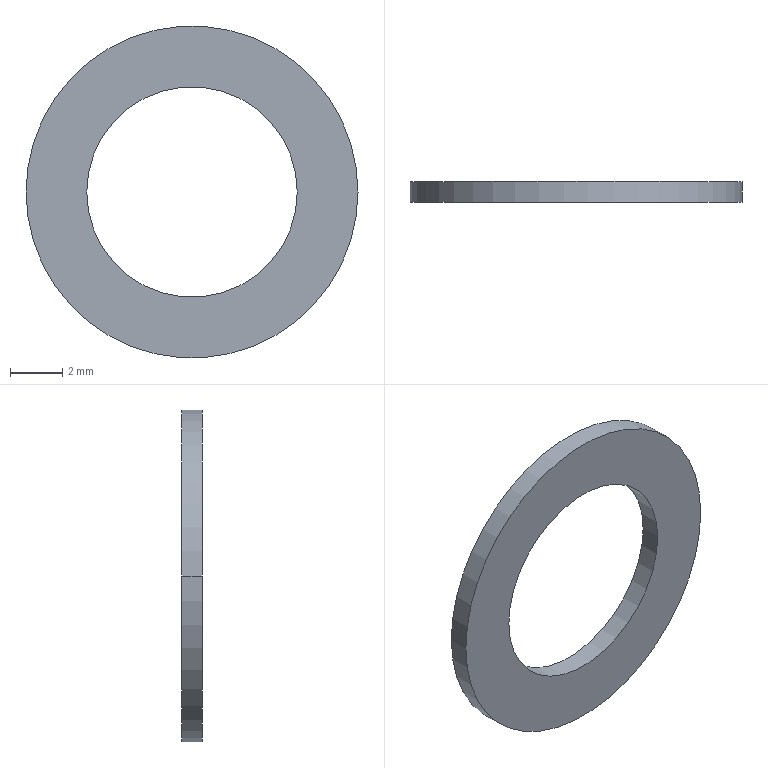Part | NX | features BREP 1 | 1 solid | 6 faces | box 12.7 x 0.7874 x 12.7 mm | volume 59.652 mm3 | cylinder 4 | plane 2 | commonest cylinder face diameters 8.052 x2 12.7 x2
STEP:
#1=CARTESIAN_POINT('',(-6.35,0.,0.));
#2=VERTEX_POINT('',#1);
#3=CARTESIAN_POINT('',(6.35,0.,0.));
#4=VERTEX_POINT('',#3);
#5=CARTESIAN_POINT('',(0.,0.,0.));
#6=DIRECTION('',(0.,1.,0.));
#7=DIRECTION('',(-1.,0.,0.));
#8=AXIS2_PLACEMENT_3D('',#5,#6,#7);
#9=CIRCLE('',#8,6.35);
#10=EDGE_CURVE('',#2,#4,#9,.T.);
#11=ORIENTED_EDGE('',*,*,#10,.F.);
#12=CARTESIAN_POINT('',(0.,0.,0.));
#13=DIRECTION('',(0.,1.,0.));
#14=DIRECTION('',(1.,0.,0.));
#15=AXIS2_PLACEMENT_3D('',#12,#13,#14);
#16=CIRCLE('',#15,6.35);
#17=EDGE_CURVE('',#4,#2,#16,.T.);
#18=ORIENTED_EDGE('',*,*,#17,.F.);
#19=EDGE_LOOP('',(#11,#18));
#20=FACE_BOUND('',#19,.T.);
#21=CARTESIAN_POINT('',(-4.026,0.,0.));
#22=VERTEX_POINT('',#21);
#23=CARTESIAN_POINT('',(4.026,0.,0.));
#24=VERTEX_POINT('',#23);
#25=CARTESIAN_POINT('',(0.,0.,0.));
#26=DIRECTION('',(0.,-1.,0.));
#27=DIRECTION('',(-1.,0.,0.));
#28=AXIS2_PLACEMENT_3D('',#25,#26,#27);
#29=CIRCLE('',#28,4.026);
#30=EDGE_CURVE('',#22,#24,#29,.T.);
#31=ORIENTED_EDGE('',*,*,#30,.F.);
#32=CARTESIAN_POINT('',(0.,0.,0.));
#33=DIRECTION('',(0.,-1.,0.));
#34=DIRECTION('',(1.,0.,0.));
#35=AXIS2_PLACEMENT_3D('',#32,#33,#34);
#36=CIRCLE('',#35,4.026);
#37=EDGE_CURVE('',#24,#22,#36,.T.);
#38=ORIENTED_EDGE('',*,*,#37,.F.);
#39=EDGE_LOOP('',(#31,#38));
#40=FACE_BOUND('',#39,.T.);
#41=CARTESIAN_POINT('',(0.,0.,0.));
#42=DIRECTION('',(0.,1.,0.));
#43=DIRECTION('',(1.,0.,0.));
#44=AXIS2_PLACEMENT_3D('',#41,#42,#43);
#45=PLANE('',#44);
#46=ADVANCED_FACE('',(#20,#40),#45,.F.);
#47=CARTESIAN_POINT('',(-6.35,0.7874,0.));
#48=VERTEX_POINT('',#47);
#49=CARTESIAN_POINT('',(-6.35,0.,0.));
#50=DIRECTION('',(0.,1.,0.));
#51=VECTOR('',#50,1000.);
#52=LINE('',#49,#51);
#53=EDGE_CURVE('',#2,#48,#52,.T.);
#54=ORIENTED_EDGE('',*,*,#53,.T.);
#55=CARTESIAN_POINT('',(6.35,0.7874,0.));
#56=VERTEX_POINT('',#55);
#57=CARTESIAN_POINT('',(0.,0.7874,0.));
#58=DIRECTION('',(0.,1.,0.));
#59=DIRECTION('',(1.,0.,0.));
#60=AXIS2_PLACEMENT_3D('',#57,#58,#59);
#61=CIRCLE('',#60,6.35);
#62=EDGE_CURVE('',#56,#48,#61,.T.);
#63=ORIENTED_EDGE('',*,*,#62,.F.);
#64=CARTESIAN_POINT('',(6.35,0.,0.));
#65=DIRECTION('',(0.,1.,0.));
#66=VECTOR('',#65,1000.);
#67=LINE('',#64,#66);
#68=EDGE_CURVE('',#4,#56,#67,.T.);
#69=ORIENTED_EDGE('',*,*,#68,.F.);
#70=ORIENTED_EDGE('',*,*,#17,.T.);
#71=EDGE_LOOP('',(#54,#63,#69,#70));
#72=FACE_BOUND('',#71,.T.);
#73=CARTESIAN_POINT('',(0.,0.,0.));
#74=DIRECTION('',(0.,1.,0.));
#75=DIRECTION('',(1.,0.,0.));
#76=AXIS2_PLACEMENT_3D('',#73,#74,#75);
#77=CYLINDRICAL_SURFACE('',#76,6.35);
#78=ADVANCED_FACE('',(#72),#77,.T.);
#79=ORIENTED_EDGE('',*,*,#68,.T.);
#80=CARTESIAN_POINT('',(0.,0.7874,0.));
#81=DIRECTION('',(0.,1.,0.));
#82=DIRECTION('',(-1.,0.,0.));
#83=AXIS2_PLACEMENT_3D('',#80,#81,#82);
#84=CIRCLE('',#83,6.35);
#85=EDGE_CURVE('',#48,#56,#84,.T.);
#86=ORIENTED_EDGE('',*,*,#85,.F.);
#87=ORIENTED_EDGE('',*,*,#53,.F.);
#88=ORIENTED_EDGE('',*,*,#10,.T.);
#89=EDGE_LOOP('',(#79,#86,#87,#88));
#90=FACE_BOUND('',#89,.T.);
#91=CARTESIAN_POINT('',(0.,0.,0.));
#92=DIRECTION('',(0.,1.,0.));
#93=DIRECTION('',(1.,0.,0.));
#94=AXIS2_PLACEMENT_3D('',#91,#92,#93);
#95=CYLINDRICAL_SURFACE('',#94,6.35);
#96=ADVANCED_FACE('',(#90),#95,.T.);
#97=ORIENTED_EDGE('',*,*,#85,.T.);
#98=ORIENTED_EDGE('',*,*,#62,.T.);
#99=EDGE_LOOP('',(#97,#98));
#100=FACE_BOUND('',#99,.T.);
#101=CARTESIAN_POINT('',(-4.026,0.7874,0.));
#102=VERTEX_POINT('',#101);
#103=CARTESIAN_POINT('',(4.026,0.7874,0.));
#104=VERTEX_POINT('',#103);
#105=CARTESIAN_POINT('',(0.,0.7874,0.));
#106=DIRECTION('',(0.,-1.,0.));
#107=DIRECTION('',(-1.,0.,0.));
#108=AXIS2_PLACEMENT_3D('',#105,#106,#107);
#109=CIRCLE('',#108,4.026);
#110=EDGE_CURVE('',#102,#104,#109,.T.);
#111=ORIENTED_EDGE('',*,*,#110,.T.);
#112=CARTESIAN_POINT('',(0.,0.7874,0.));
#113=DIRECTION('',(0.,-1.,0.));
#114=DIRECTION('',(1.,0.,0.));
#115=AXIS2_PLACEMENT_3D('',#112,#113,#114);
#116=CIRCLE('',#115,4.026);
#117=EDGE_CURVE('',#104,#102,#116,.T.);
#118=ORIENTED_EDGE('',*,*,#117,.T.);
#119=EDGE_LOOP('',(#111,#118));
#120=FACE_BOUND('',#119,.T.);
#121=CARTESIAN_POINT('',(0.,0.7874,0.));
#122=DIRECTION('',(0.,1.,0.));
#123=DIRECTION('',(1.,0.,0.));
#124=AXIS2_PLACEMENT_3D('',#121,#122,#123);
#125=PLANE('',#124);
#126=ADVANCED_FACE('',(#100,#120),#125,.T.);
#127=CARTESIAN_POINT('',(-4.026,0.7874,0.));
#128=DIRECTION('',(0.,-1.,0.));
#129=VECTOR('',#128,1000.);
#130=LINE('',#127,#129);
#131=EDGE_CURVE('',#102,#22,#130,.T.);
#132=ORIENTED_EDGE('',*,*,#131,.F.);
#133=ORIENTED_EDGE('',*,*,#117,.F.);
#134=CARTESIAN_POINT('',(4.026,0.7874,0.));
#135=DIRECTION('',(0.,-1.,0.));
#136=VECTOR('',#135,1000.);
#137=LINE('',#134,#136);
#138=EDGE_CURVE('',#104,#24,#137,.T.);
#139=ORIENTED_EDGE('',*,*,#138,.T.);
#140=ORIENTED_EDGE('',*,*,#37,.T.);
#141=EDGE_LOOP('',(#132,#133,#139,#140));
#142=FACE_BOUND('',#141,.T.);
#143=CARTESIAN_POINT('',(0.,0.7874,0.));
#144=DIRECTION('',(0.,-1.,0.));
#145=DIRECTION('',(1.,0.,0.));
#146=AXIS2_PLACEMENT_3D('',#143,#144,#145);
#147=CYLINDRICAL_SURFACE('',#146,4.026);
#148=ADVANCED_FACE('',(#142),#147,.F.);
#149=ORIENTED_EDGE('',*,*,#138,.F.);
#150=ORIENTED_EDGE('',*,*,#110,.F.);
#151=ORIENTED_EDGE('',*,*,#131,.T.);
#152=ORIENTED_EDGE('',*,*,#30,.T.);
#153=EDGE_LOOP('',(#149,#150,#151,#152));
#154=FACE_BOUND('',#153,.T.);
#155=CARTESIAN_POINT('',(0.,0.7874,0.));
#156=DIRECTION('',(0.,-1.,0.));
#157=DIRECTION('',(1.,0.,0.));
#158=AXIS2_PLACEMENT_3D('',#155,#156,#157);
#159=CYLINDRICAL_SURFACE('',#158,4.026);
#160=ADVANCED_FACE('',(#154),#159,.F.);
#161=CLOSED_SHELL('',(#46,#78,#96,#126,#148,#160));
#162=MANIFOLD_SOLID_BREP('',#161);
#163=(LENGTH_UNIT()NAMED_UNIT(*)SI_UNIT(.MILLI.,.METRE.));
#164=UNCERTAINTY_MEASURE_WITH_UNIT(LENGTH_MEASURE(0.00001),#163,'','');
#165=(NAMED_UNIT(*)PLANE_ANGLE_UNIT()SI_UNIT($,.RADIAN.));
#166=(NAMED_UNIT(*)SI_UNIT($,.STERADIAN.)SOLID_ANGLE_UNIT());
#167=(GEOMETRIC_REPRESENTATION_CONTEXT(3)GLOBAL_UNCERTAINTY_ASSIGNED_CONTEXT((#164))GLOBAL_UNIT_ASSIGNED_CONTEXT((#163,#165,#166))REPRESENTATION_CONTEXT('',''));
#168=ADVANCED_BREP_SHAPE_REPRESENTATION('',(#162),#167);